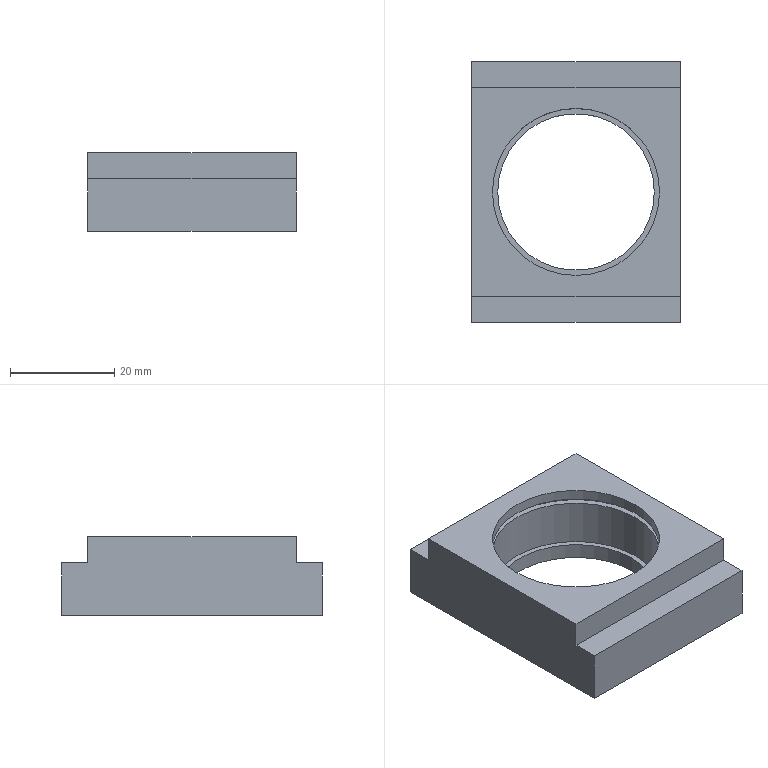Part | STEP file | Bearing fixing seat | 1 solid | 21 faces | box 40 x 50 x 15 mm | volume 16103 mm3 | plane 13 | cylinder 8 | commonest cylinder face diameters 32 x4 30 x2 34.4 x2
STEP:
#1=CARTESIAN_POINT('',(0.,0.,0.));
#2=DIRECTION('',(0.,0.,1.));
#3=DIRECTION('',(1.,0.,0.));
#4=AXIS2_PLACEMENT_3D('',#1,#2,#3);
#5=CARTESIAN_POINT('',(15.,0.,0.));
#6=VERTEX_POINT('',#5);
#7=CARTESIAN_POINT('',(15.,0.,3.));
#8=VERTEX_POINT('',#7);
#9=CARTESIAN_POINT('',(15.,0.,-3.));
#10=DIRECTION('',(0.,0.,1.));
#11=VECTOR('',#10,1.);
#12=LINE('',#9,#11);
#13=CARTESIAN_POINT('',(0.,0.,-3.));
#14=DIRECTION('',(0.,0.,1.));
#15=DIRECTION('',(1.,0.,0.));
#16=AXIS2_PLACEMENT_3D('',#13,#14,#15);
#17=CYLINDRICAL_SURFACE('',#16,15.);
#18=CARTESIAN_POINT('',(6.283,0.));
#19=DIRECTION('',(0.,1.));
#20=VECTOR('',#19,1.);
#21=LINE('',#18,#20);
#22=(GEOMETRIC_REPRESENTATION_CONTEXT(2)PARAMETRIC_REPRESENTATION_CONTEXT()REPRESENTATION_CONTEXT('',''));
#23=DEFINITIONAL_REPRESENTATION('',(#21),#22);
#24=PCURVE('',#17,#23);
#25=CARTESIAN_POINT('',(0.,0.,-3.));
#26=DIRECTION('',(0.,0.,1.));
#27=DIRECTION('',(1.,0.,0.));
#28=AXIS2_PLACEMENT_3D('',#25,#26,#27);
#29=CYLINDRICAL_SURFACE('',#28,15.);
#30=CARTESIAN_POINT('',(0.,0.));
#31=DIRECTION('',(0.,1.));
#32=VECTOR('',#31,1.);
#33=LINE('',#30,#32);
#34=(GEOMETRIC_REPRESENTATION_CONTEXT(2)PARAMETRIC_REPRESENTATION_CONTEXT()REPRESENTATION_CONTEXT('',''));
#35=DEFINITIONAL_REPRESENTATION('',(#33),#34);
#36=PCURVE('',#29,#35);
#37=SURFACE_CURVE('',#12,(#24,#36),.PCURVE_S1.);
#38=EDGE_CURVE('',#6,#8,#37,.T.);
#39=ORIENTED_EDGE('',*,*,#38,.T.);
#40=CARTESIAN_POINT('',(-15.,0.,3.));
#41=VERTEX_POINT('',#40);
#42=CARTESIAN_POINT('',(0.,0.,3.));
#43=DIRECTION('',(0.,0.,-1.));
#44=DIRECTION('',(1.,0.,0.));
#45=AXIS2_PLACEMENT_3D('',#42,#43,#44);
#46=CIRCLE('',#45,15.);
#47=CARTESIAN_POINT('',(6.283,6.));
#48=DIRECTION('',(-1.,0.));
#49=VECTOR('',#48,1.);
#50=LINE('',#47,#49);
#51=(GEOMETRIC_REPRESENTATION_CONTEXT(2)PARAMETRIC_REPRESENTATION_CONTEXT()REPRESENTATION_CONTEXT('',''));
#52=DEFINITIONAL_REPRESENTATION('',(#50),#51);
#53=PCURVE('',#17,#52);
#54=CARTESIAN_POINT('',(0.,0.,3.));
#55=DIRECTION('',(0.,0.,1.));
#56=DIRECTION('',(1.,0.,0.));
#57=AXIS2_PLACEMENT_3D('',#54,#55,#56);
#58=PLANE('',#57);
#59=CARTESIAN_POINT('',(15.,0.));
#60=CARTESIAN_POINT('',(15.,-25.981));
#61=CARTESIAN_POINT('',(-7.5,-12.99));
#62=CARTESIAN_POINT('',(-30.,0.));
#63=CARTESIAN_POINT('',(-7.5,12.99));
#64=CARTESIAN_POINT('',(15.,25.981));
#65=CARTESIAN_POINT('',(15.,0.));
#66=(BOUNDED_CURVE()B_SPLINE_CURVE(2,(#59,#60,#61,#62,#63,#64,#65),.UNSPECIFIED.,.T.,.F.)B_SPLINE_CURVE_WITH_KNOTS((1,2,2,2,2,1),(-2.094,0.,2.094,4.189,6.283,8.378),.UNSPECIFIED.)CURVE()GEOMETRIC_REPRESENTATION_ITEM()RATIONAL_B_SPLINE_CURVE((1.,0.5,1.,0.5,1.,0.5,1.))REPRESENTATION_ITEM(''));
#67=(GEOMETRIC_REPRESENTATION_CONTEXT(2)PARAMETRIC_REPRESENTATION_CONTEXT()REPRESENTATION_CONTEXT('',''));
#68=DEFINITIONAL_REPRESENTATION('',(#66),#67);
#69=PCURVE('',#58,#68);
#70=SURFACE_CURVE('',#46,(#53,#69),.PCURVE_S1.);
#71=EDGE_CURVE('',#8,#41,#70,.T.);
#72=ORIENTED_EDGE('',*,*,#71,.T.);
#73=CARTESIAN_POINT('',(-15.,0.,0.));
#74=VERTEX_POINT('',#73);
#75=CARTESIAN_POINT('',(-15.,0.,-3.));
#76=DIRECTION('',(0.,0.,1.));
#77=VECTOR('',#76,1.);
#78=LINE('',#75,#77);
#79=CARTESIAN_POINT('',(3.142,0.));
#80=DIRECTION('',(0.,1.));
#81=VECTOR('',#80,1.);
#82=LINE('',#79,#81);
#83=(GEOMETRIC_REPRESENTATION_CONTEXT(2)PARAMETRIC_REPRESENTATION_CONTEXT()REPRESENTATION_CONTEXT('',''));
#84=DEFINITIONAL_REPRESENTATION('',(#82),#83);
#85=PCURVE('',#17,#84);
#86=CARTESIAN_POINT('',(3.142,0.));
#87=DIRECTION('',(0.,1.));
#88=VECTOR('',#87,1.);
#89=LINE('',#86,#88);
#90=(GEOMETRIC_REPRESENTATION_CONTEXT(2)PARAMETRIC_REPRESENTATION_CONTEXT()REPRESENTATION_CONTEXT('',''));
#91=DEFINITIONAL_REPRESENTATION('',(#89),#90);
#92=PCURVE('',#29,#91);
#93=SURFACE_CURVE('',#78,(#85,#92),.PCURVE_S1.);
#94=EDGE_CURVE('',#74,#41,#93,.T.);
#95=ORIENTED_EDGE('',*,*,#94,.F.);
#96=CARTESIAN_POINT('',(0.,0.,0.));
#97=DIRECTION('',(0.,0.,-1.));
#98=DIRECTION('',(1.,0.,0.));
#99=AXIS2_PLACEMENT_3D('',#96,#97,#98);
#100=CIRCLE('',#99,15.);
#101=CARTESIAN_POINT('',(6.283,3.));
#102=DIRECTION('',(-1.,0.));
#103=VECTOR('',#102,1.);
#104=LINE('',#101,#103);
#105=(GEOMETRIC_REPRESENTATION_CONTEXT(2)PARAMETRIC_REPRESENTATION_CONTEXT()REPRESENTATION_CONTEXT('',''));
#106=DEFINITIONAL_REPRESENTATION('',(#104),#105);
#107=PCURVE('',#17,#106);
#108=CARTESIAN_POINT('',(0.,0.,0.));
#109=DIRECTION('',(0.,0.,1.));
#110=DIRECTION('',(1.,0.,0.));
#111=AXIS2_PLACEMENT_3D('',#108,#109,#110);
#112=PLANE('',#111);
#113=CARTESIAN_POINT('',(15.,0.));
#114=CARTESIAN_POINT('',(15.,-25.981));
#115=CARTESIAN_POINT('',(-7.5,-12.99));
#116=CARTESIAN_POINT('',(-30.,0.));
#117=CARTESIAN_POINT('',(-7.5,12.99));
#118=CARTESIAN_POINT('',(15.,25.981));
#119=CARTESIAN_POINT('',(15.,0.));
#120=(BOUNDED_CURVE()B_SPLINE_CURVE(2,(#113,#114,#115,#116,#117,#118,#119),.UNSPECIFIED.,.T.,.F.)B_SPLINE_CURVE_WITH_KNOTS((1,2,2,2,2,1),(-2.094,0.,2.094,4.189,6.283,8.378),.UNSPECIFIED.)CURVE()GEOMETRIC_REPRESENTATION_ITEM()RATIONAL_B_SPLINE_CURVE((1.,0.5,1.,0.5,1.,0.5,1.))REPRESENTATION_ITEM(''));
#121=(GEOMETRIC_REPRESENTATION_CONTEXT(2)PARAMETRIC_REPRESENTATION_CONTEXT()REPRESENTATION_CONTEXT('',''));
#122=DEFINITIONAL_REPRESENTATION('',(#120),#121);
#123=PCURVE('',#112,#122);
#124=SURFACE_CURVE('',#100,(#107,#123),.PCURVE_S1.);
#125=EDGE_CURVE('',#6,#74,#124,.T.);
#126=ORIENTED_EDGE('',*,*,#125,.F.);
#127=EDGE_LOOP('',(#39,#72,#95,#126));
#128=FACE_BOUND('',#127,.F.);
#129=ADVANCED_FACE('',(#128),#17,.F.);
#130=CARTESIAN_POINT('',(-16.,0.,15.));
#131=VERTEX_POINT('',#130);
#132=CARTESIAN_POINT('',(-16.,0.,13.));
#133=VERTEX_POINT('',#132);
#134=CARTESIAN_POINT('',(-16.,0.,15.));
#135=DIRECTION('',(0.,0.,-1.));
#136=VECTOR('',#135,1.);
#137=LINE('',#134,#136);
#138=CARTESIAN_POINT('',(0.,0.,15.));
#139=DIRECTION('',(0.,0.,-1.));
#140=DIRECTION('',(-1.,0.,0.));
#141=AXIS2_PLACEMENT_3D('',#138,#139,#140);
#142=CYLINDRICAL_SURFACE('',#141,16.);
#143=CARTESIAN_POINT('',(6.283,0.));
#144=DIRECTION('',(0.,1.));
#145=VECTOR('',#144,1.);
#146=LINE('',#143,#145);
#147=(GEOMETRIC_REPRESENTATION_CONTEXT(2)PARAMETRIC_REPRESENTATION_CONTEXT()REPRESENTATION_CONTEXT('',''));
#148=DEFINITIONAL_REPRESENTATION('',(#146),#147);
#149=PCURVE('',#142,#148);
#150=CARTESIAN_POINT('',(0.,0.,15.));
#151=DIRECTION('',(0.,0.,-1.));
#152=DIRECTION('',(-1.,0.,0.));
#153=AXIS2_PLACEMENT_3D('',#150,#151,#152);
#154=CYLINDRICAL_SURFACE('',#153,16.);
#155=CARTESIAN_POINT('',(0.,0.));
#156=DIRECTION('',(0.,1.));
#157=VECTOR('',#156,1.);
#158=LINE('',#155,#157);
#159=(GEOMETRIC_REPRESENTATION_CONTEXT(2)PARAMETRIC_REPRESENTATION_CONTEXT()REPRESENTATION_CONTEXT('',''));
#160=DEFINITIONAL_REPRESENTATION('',(#158),#159);
#161=PCURVE('',#154,#160);
#162=SURFACE_CURVE('',#137,(#149,#161),.PCURVE_S1.);
#163=EDGE_CURVE('',#131,#133,#162,.T.);
#164=ORIENTED_EDGE('',*,*,#163,.T.);
#165=CARTESIAN_POINT('',(16.,0.,13.));
#166=VERTEX_POINT('',#165);
#167=CARTESIAN_POINT('',(0.,0.,13.));
#168=DIRECTION('',(0.,0.,1.));
#169=DIRECTION('',(-1.,0.,0.));
#170=AXIS2_PLACEMENT_3D('',#167,#168,#169);
#171=CIRCLE('',#170,16.);
#172=CARTESIAN_POINT('',(6.283,2.));
#173=DIRECTION('',(-1.,0.));
#174=VECTOR('',#173,1.);
#175=LINE('',#172,#174);
#176=(GEOMETRIC_REPRESENTATION_CONTEXT(2)PARAMETRIC_REPRESENTATION_CONTEXT()REPRESENTATION_CONTEXT('',''));
#177=DEFINITIONAL_REPRESENTATION('',(#175),#176);
#178=PCURVE('',#142,#177);
#179=CARTESIAN_POINT('',(0.,0.,13.));
#180=DIRECTION('',(0.,0.,1.));
#181=DIRECTION('',(1.,0.,0.));
#182=AXIS2_PLACEMENT_3D('',#179,#180,#181);
#183=PLANE('',#182);
#184=CARTESIAN_POINT('',(0.,0.));
#185=DIRECTION('',(-1.,0.));
#186=AXIS2_PLACEMENT_2D('',#184,#185);
#187=CIRCLE('',#186,16.);
#188=(GEOMETRIC_REPRESENTATION_CONTEXT(2)PARAMETRIC_REPRESENTATION_CONTEXT()REPRESENTATION_CONTEXT('',''));
#189=DEFINITIONAL_REPRESENTATION('',(#187),#188);
#190=PCURVE('',#183,#189);
#191=SURFACE_CURVE('',#171,(#178,#190),.PCURVE_S1.);
#192=EDGE_CURVE('',#133,#166,#191,.T.);
#193=ORIENTED_EDGE('',*,*,#192,.T.);
#194=CARTESIAN_POINT('',(16.,0.,15.));
#195=VERTEX_POINT('',#194);
#196=CARTESIAN_POINT('',(16.,0.,15.));
#197=DIRECTION('',(0.,0.,-1.));
#198=VECTOR('',#197,1.);
#199=LINE('',#196,#198);
#200=CARTESIAN_POINT('',(3.142,0.));
#201=DIRECTION('',(0.,1.));
#202=VECTOR('',#201,1.);
#203=LINE('',#200,#202);
#204=(GEOMETRIC_REPRESENTATION_CONTEXT(2)PARAMETRIC_REPRESENTATION_CONTEXT()REPRESENTATION_CONTEXT('',''));
#205=DEFINITIONAL_REPRESENTATION('',(#203),#204);
#206=PCURVE('',#142,#205);
#207=CARTESIAN_POINT('',(3.142,0.));
#208=DIRECTION('',(0.,1.));
#209=VECTOR('',#208,1.);
#210=LINE('',#207,#209);
#211=(GEOMETRIC_REPRESENTATION_CONTEXT(2)PARAMETRIC_REPRESENTATION_CONTEXT()REPRESENTATION_CONTEXT('',''));
#212=DEFINITIONAL_REPRESENTATION('',(#210),#211);
#213=PCURVE('',#154,#212);
#214=SURFACE_CURVE('',#199,(#206,#213),.PCURVE_S1.);
#215=EDGE_CURVE('',#195,#166,#214,.T.);
#216=ORIENTED_EDGE('',*,*,#215,.F.);
#217=CARTESIAN_POINT('',(0.,0.,15.));
#218=DIRECTION('',(0.,0.,-1.));
#219=DIRECTION('',(-1.,0.,0.));
#220=AXIS2_PLACEMENT_3D('',#217,#218,#219);
#221=CIRCLE('',#220,16.);
#222=CARTESIAN_POINT('',(0.,0.));
#223=DIRECTION('',(1.,0.));
#224=VECTOR('',#223,1.);
#225=LINE('',#222,#224);
#226=(GEOMETRIC_REPRESENTATION_CONTEXT(2)PARAMETRIC_REPRESENTATION_CONTEXT()REPRESENTATION_CONTEXT('',''));
#227=DEFINITIONAL_REPRESENTATION('',(#225),#226);
#228=PCURVE('',#142,#227);
#229=CARTESIAN_POINT('',(0.,0.,15.));
#230=DIRECTION('',(0.,0.,1.));
#231=DIRECTION('',(1.,0.,0.));
#232=AXIS2_PLACEMENT_3D('',#229,#230,#231);
#233=PLANE('',#232);
#234=CARTESIAN_POINT('',(-16.,0.));
#235=CARTESIAN_POINT('',(-16.,27.713));
#236=CARTESIAN_POINT('',(8.,13.856));
#237=CARTESIAN_POINT('',(32.,0.));
#238=CARTESIAN_POINT('',(8.,-13.856));
#239=CARTESIAN_POINT('',(-16.,-27.713));
#240=CARTESIAN_POINT('',(-16.,0.));
#241=(BOUNDED_CURVE()B_SPLINE_CURVE(2,(#234,#235,#236,#237,#238,#239,#240),.UNSPECIFIED.,.T.,.F.)B_SPLINE_CURVE_WITH_KNOTS((1,2,2,2,2,1),(-2.094,0.,2.094,4.189,6.283,8.378),.UNSPECIFIED.)CURVE()GEOMETRIC_REPRESENTATION_ITEM()RATIONAL_B_SPLINE_CURVE((1.,0.5,1.,0.5,1.,0.5,1.))REPRESENTATION_ITEM(''));
#242=(GEOMETRIC_REPRESENTATION_CONTEXT(2)PARAMETRIC_REPRESENTATION_CONTEXT()REPRESENTATION_CONTEXT('',''));
#243=DEFINITIONAL_REPRESENTATION('',(#241),#242);
#244=PCURVE('',#233,#243);
#245=SURFACE_CURVE('',#221,(#228,#244),.PCURVE_S1.);
#246=EDGE_CURVE('',#195,#131,#245,.T.);
#247=ORIENTED_EDGE('',*,*,#246,.T.);
#248=EDGE_LOOP('',(#164,#193,#216,#247));
#249=FACE_BOUND('',#248,.F.);
#250=ADVANCED_FACE('',(#249),#142,.F.);
#251=CARTESIAN_POINT('',(16.,0.,3.));
#252=VERTEX_POINT('',#251);
#253=CARTESIAN_POINT('',(16.,0.,12.));
#254=VERTEX_POINT('',#253);
#255=CARTESIAN_POINT('',(16.,0.,3.));
#256=DIRECTION('',(0.,0.,1.));
#257=VECTOR('',#256,1.);
#258=LINE('',#255,#257);
#259=CARTESIAN_POINT('',(0.,0.,3.));
#260=DIRECTION('',(0.,0.,1.));
#261=DIRECTION('',(1.,0.,0.));
#262=AXIS2_PLACEMENT_3D('',#259,#260,#261);
#263=CYLINDRICAL_SURFACE('',#262,16.);
#264=CARTESIAN_POINT('',(6.283,0.));
#265=DIRECTION('',(0.,1.));
#266=VECTOR('',#265,1.);
#267=LINE('',#264,#266);
#268=(GEOMETRIC_REPRESENTATION_CONTEXT(2)PARAMETRIC_REPRESENTATION_CONTEXT()REPRESENTATION_CONTEXT('',''));
#269=DEFINITIONAL_REPRESENTATION('',(#267),#268);
#270=PCURVE('',#263,#269);
#271=CARTESIAN_POINT('',(0.,0.,3.));
#272=DIRECTION('',(0.,0.,1.));
#273=DIRECTION('',(1.,0.,0.));
#274=AXIS2_PLACEMENT_3D('',#271,#272,#273);
#275=CYLINDRICAL_SURFACE('',#274,16.);
#276=CARTESIAN_POINT('',(0.,0.));
#277=DIRECTION('',(0.,1.));
#278=VECTOR('',#277,1.);
#279=LINE('',#276,#278);
#280=(GEOMETRIC_REPRESENTATION_CONTEXT(2)PARAMETRIC_REPRESENTATION_CONTEXT()REPRESENTATION_CONTEXT('',''));
#281=DEFINITIONAL_REPRESENTATION('',(#279),#280);
#282=PCURVE('',#275,#281);
#283=SURFACE_CURVE('',#258,(#270,#282),.PCURVE_S1.);
#284=EDGE_CURVE('',#252,#254,#283,.T.);
#285=ORIENTED_EDGE('',*,*,#284,.T.);
#286=CARTESIAN_POINT('',(-16.,0.,12.));
#287=VERTEX_POINT('',#286);
#288=CARTESIAN_POINT('',(0.,0.,12.));
#289=DIRECTION('',(0.,0.,-1.));
#290=DIRECTION('',(1.,0.,0.));
#291=AXIS2_PLACEMENT_3D('',#288,#289,#290);
#292=CIRCLE('',#291,16.);
#293=CARTESIAN_POINT('',(6.283,9.));
#294=DIRECTION('',(-1.,0.));
#295=VECTOR('',#294,1.);
#296=LINE('',#293,#295);
#297=(GEOMETRIC_REPRESENTATION_CONTEXT(2)PARAMETRIC_REPRESENTATION_CONTEXT()REPRESENTATION_CONTEXT('',''));
#298=DEFINITIONAL_REPRESENTATION('',(#296),#297);
#299=PCURVE('',#263,#298);
#300=CARTESIAN_POINT('',(0.,0.,12.));
#301=DIRECTION('',(0.,0.,1.));
#302=DIRECTION('',(1.,0.,0.));
#303=AXIS2_PLACEMENT_3D('',#300,#301,#302);
#304=PLANE('',#303);
#305=CARTESIAN_POINT('',(16.,0.));
#306=CARTESIAN_POINT('',(16.,-27.713));
#307=CARTESIAN_POINT('',(-8.,-13.856));
#308=CARTESIAN_POINT('',(-32.,0.));
#309=CARTESIAN_POINT('',(-8.,13.856));
#310=CARTESIAN_POINT('',(16.,27.713));
#311=CARTESIAN_POINT('',(16.,0.));
#312=(BOUNDED_CURVE()B_SPLINE_CURVE(2,(#305,#306,#307,#308,#309,#310,#311),.UNSPECIFIED.,.T.,.F.)B_SPLINE_CURVE_WITH_KNOTS((1,2,2,2,2,1),(-2.094,0.,2.094,4.189,6.283,8.378),.UNSPECIFIED.)CURVE()GEOMETRIC_REPRESENTATION_ITEM()RATIONAL_B_SPLINE_CURVE((1.,0.5,1.,0.5,1.,0.5,1.))REPRESENTATION_ITEM(''));
#313=(GEOMETRIC_REPRESENTATION_CONTEXT(2)PARAMETRIC_REPRESENTATION_CONTEXT()REPRESENTATION_CONTEXT('',''));
#314=DEFINITIONAL_REPRESENTATION('',(#312),#313);
#315=PCURVE('',#304,#314);
#316=SURFACE_CURVE('',#292,(#299,#315),.PCURVE_S1.);
#317=EDGE_CURVE('',#254,#287,#316,.T.);
#318=ORIENTED_EDGE('',*,*,#317,.T.);
#319=CARTESIAN_POINT('',(-16.,0.,3.));
#320=VERTEX_POINT('',#319);
#321=CARTESIAN_POINT('',(-16.,0.,3.));
#322=DIRECTION('',(0.,0.,1.));
#323=VECTOR('',#322,1.);
#324=LINE('',#321,#323);
#325=CARTESIAN_POINT('',(3.142,0.));
#326=DIRECTION('',(0.,1.));
#327=VECTOR('',#326,1.);
#328=LINE('',#325,#327);
#329=(GEOMETRIC_REPRESENTATION_CONTEXT(2)PARAMETRIC_REPRESENTATION_CONTEXT()REPRESENTATION_CONTEXT('',''));
#330=DEFINITIONAL_REPRESENTATION('',(#328),#329);
#331=PCURVE('',#263,#330);
#332=CARTESIAN_POINT('',(3.142,0.));
#333=DIRECTION('',(0.,1.));
#334=VECTOR('',#333,1.);
#335=LINE('',#332,#334);
#336=(GEOMETRIC_REPRESENTATION_CONTEXT(2)PARAMETRIC_REPRESENTATION_CONTEXT()REPRESENTATION_CONTEXT('',''));
#337=DEFINITIONAL_REPRESENTATION('',(#335),#336);
#338=PCURVE('',#275,#337);
#339=SURFACE_CURVE('',#324,(#331,#338),.PCURVE_S1.);
#340=EDGE_CURVE('',#320,#287,#339,.T.);
#341=ORIENTED_EDGE('',*,*,#340,.F.);
#342=CARTESIAN_POINT('',(0.,0.,3.));
#343=DIRECTION('',(0.,0.,1.));
#344=DIRECTION('',(1.,0.,0.));
#345=AXIS2_PLACEMENT_3D('',#342,#343,#344);
#346=CIRCLE('',#345,16.);
#347=CARTESIAN_POINT('',(0.,0.));
#348=DIRECTION('',(1.,0.));
#349=VECTOR('',#348,1.);
#350=LINE('',#347,#349);
#351=(GEOMETRIC_REPRESENTATION_CONTEXT(2)PARAMETRIC_REPRESENTATION_CONTEXT()REPRESENTATION_CONTEXT('',''));
#352=DEFINITIONAL_REPRESENTATION('',(#350),#351);
#353=PCURVE('',#263,#352);
#354=CARTESIAN_POINT('',(0.,0.));
#355=DIRECTION('',(1.,0.));
#356=AXIS2_PLACEMENT_2D('',#354,#355);
#357=CIRCLE('',#356,16.);
#358=(GEOMETRIC_REPRESENTATION_CONTEXT(2)PARAMETRIC_REPRESENTATION_CONTEXT()REPRESENTATION_CONTEXT('',''));
#359=DEFINITIONAL_REPRESENTATION('',(#357),#358);
#360=PCURVE('',#58,#359);
#361=SURFACE_CURVE('',#346,(#353,#360),.PCURVE_S1.);
#362=EDGE_CURVE('',#320,#252,#361,.T.);
#363=ORIENTED_EDGE('',*,*,#362,.T.);
#364=EDGE_LOOP('',(#285,#318,#341,#363));
#365=FACE_BOUND('',#364,.F.);
#366=ADVANCED_FACE('',(#365),#263,.F.);
#367=CARTESIAN_POINT('',(-17.2,0.,13.));
#368=VERTEX_POINT('',#367);
#369=CARTESIAN_POINT('',(-17.2,0.,12.));
#370=VERTEX_POINT('',#369);
#371=CARTESIAN_POINT('',(-17.2,0.,13.));
#372=DIRECTION('',(0.,0.,-1.));
#373=VECTOR('',#372,1.);
#374=LINE('',#371,#373);
#375=CARTESIAN_POINT('',(0.,0.,13.));
#376=DIRECTION('',(0.,0.,-1.));
#377=DIRECTION('',(-1.,0.,0.));
#378=AXIS2_PLACEMENT_3D('',#375,#376,#377);
#379=CYLINDRICAL_SURFACE('',#378,17.2);
#380=CARTESIAN_POINT('',(6.283,0.));
#381=DIRECTION('',(0.,1.));
#382=VECTOR('',#381,1.);
#383=LINE('',#380,#382);
#384=(GEOMETRIC_REPRESENTATION_CONTEXT(2)PARAMETRIC_REPRESENTATION_CONTEXT()REPRESENTATION_CONTEXT('',''));
#385=DEFINITIONAL_REPRESENTATION('',(#383),#384);
#386=PCURVE('',#379,#385);
#387=CARTESIAN_POINT('',(0.,0.,13.));
#388=DIRECTION('',(0.,0.,-1.));
#389=DIRECTION('',(-1.,0.,0.));
#390=AXIS2_PLACEMENT_3D('',#387,#388,#389);
#391=CYLINDRICAL_SURFACE('',#390,17.2);
#392=CARTESIAN_POINT('',(0.,0.));
#393=DIRECTION('',(0.,1.));
#394=VECTOR('',#393,1.);
#395=LINE('',#392,#394);
#396=(GEOMETRIC_REPRESENTATION_CONTEXT(2)PARAMETRIC_REPRESENTATION_CONTEXT()REPRESENTATION_CONTEXT('',''));
#397=DEFINITIONAL_REPRESENTATION('',(#395),#396);
#398=PCURVE('',#391,#397);
#399=SURFACE_CURVE('',#374,(#386,#398),.PCURVE_S1.);
#400=EDGE_CURVE('',#368,#370,#399,.T.);
#401=ORIENTED_EDGE('',*,*,#400,.T.);
#402=CARTESIAN_POINT('',(17.2,0.,12.));
#403=VERTEX_POINT('',#402);
#404=CARTESIAN_POINT('',(0.,0.,12.));
#405=DIRECTION('',(0.,0.,1.));
#406=DIRECTION('',(-1.,0.,0.));
#407=AXIS2_PLACEMENT_3D('',#404,#405,#406);
#408=CIRCLE('',#407,17.2);
#409=CARTESIAN_POINT('',(6.283,1.));
#410=DIRECTION('',(-1.,0.));
#411=VECTOR('',#410,1.);
#412=LINE('',#409,#411);
#413=(GEOMETRIC_REPRESENTATION_CONTEXT(2)PARAMETRIC_REPRESENTATION_CONTEXT()REPRESENTATION_CONTEXT('',''));
#414=DEFINITIONAL_REPRESENTATION('',(#412),#413);
#415=PCURVE('',#379,#414);
#416=CARTESIAN_POINT('',(0.,0.));
#417=DIRECTION('',(-1.,0.));
#418=AXIS2_PLACEMENT_2D('',#416,#417);
#419=CIRCLE('',#418,17.2);
#420=(GEOMETRIC_REPRESENTATION_CONTEXT(2)PARAMETRIC_REPRESENTATION_CONTEXT()REPRESENTATION_CONTEXT('',''));
#421=DEFINITIONAL_REPRESENTATION('',(#419),#420);
#422=PCURVE('',#304,#421);
#423=SURFACE_CURVE('',#408,(#415,#422),.PCURVE_S1.);
#424=EDGE_CURVE('',#370,#403,#423,.T.);
#425=ORIENTED_EDGE('',*,*,#424,.T.);
#426=CARTESIAN_POINT('',(17.2,0.,13.));
#427=VERTEX_POINT('',#426);
#428=CARTESIAN_POINT('',(17.2,0.,13.));
#429=DIRECTION('',(0.,0.,-1.));
#430=VECTOR('',#429,1.);
#431=LINE('',#428,#430);
#432=CARTESIAN_POINT('',(3.142,0.));
#433=DIRECTION('',(0.,1.));
#434=VECTOR('',#433,1.);
#435=LINE('',#432,#434);
#436=(GEOMETRIC_REPRESENTATION_CONTEXT(2)PARAMETRIC_REPRESENTATION_CONTEXT()REPRESENTATION_CONTEXT('',''));
#437=DEFINITIONAL_REPRESENTATION('',(#435),#436);
#438=PCURVE('',#379,#437);
#439=CARTESIAN_POINT('',(3.142,0.));
#440=DIRECTION('',(0.,1.));
#441=VECTOR('',#440,1.);
#442=LINE('',#439,#441);
#443=(GEOMETRIC_REPRESENTATION_CONTEXT(2)PARAMETRIC_REPRESENTATION_CONTEXT()REPRESENTATION_CONTEXT('',''));
#444=DEFINITIONAL_REPRESENTATION('',(#442),#443);
#445=PCURVE('',#391,#444);
#446=SURFACE_CURVE('',#431,(#438,#445),.PCURVE_S1.);
#447=EDGE_CURVE('',#427,#403,#446,.T.);
#448=ORIENTED_EDGE('',*,*,#447,.F.);
#449=CARTESIAN_POINT('',(0.,0.,13.));
#450=DIRECTION('',(0.,0.,1.));
#451=DIRECTION('',(-1.,0.,0.));
#452=AXIS2_PLACEMENT_3D('',#449,#450,#451);
#453=CIRCLE('',#452,17.2);
#454=CARTESIAN_POINT('',(6.283,0.));
#455=DIRECTION('',(-1.,0.));
#456=VECTOR('',#455,1.);
#457=LINE('',#454,#456);
#458=(GEOMETRIC_REPRESENTATION_CONTEXT(2)PARAMETRIC_REPRESENTATION_CONTEXT()REPRESENTATION_CONTEXT('',''));
#459=DEFINITIONAL_REPRESENTATION('',(#457),#458);
#460=PCURVE('',#379,#459);
#461=CARTESIAN_POINT('',(0.,0.));
#462=DIRECTION('',(-1.,0.));
#463=AXIS2_PLACEMENT_2D('',#461,#462);
#464=CIRCLE('',#463,17.2);
#465=(GEOMETRIC_REPRESENTATION_CONTEXT(2)PARAMETRIC_REPRESENTATION_CONTEXT()REPRESENTATION_CONTEXT('',''));
#466=DEFINITIONAL_REPRESENTATION('',(#464),#465);
#467=PCURVE('',#183,#466);
#468=SURFACE_CURVE('',#453,(#460,#467),.PCURVE_S1.);
#469=EDGE_CURVE('',#368,#427,#468,.T.);
#470=ORIENTED_EDGE('',*,*,#469,.F.);
#471=EDGE_LOOP('',(#401,#425,#448,#470));
#472=FACE_BOUND('',#471,.F.);
#473=ADVANCED_FACE('',(#472),#379,.F.);
#474=CARTESIAN_POINT('',(-20.,-25.,0.));
#475=VERTEX_POINT('',#474);
#476=CARTESIAN_POINT('',(20.,-25.,0.));
#477=VERTEX_POINT('',#476);
#478=CARTESIAN_POINT('',(0.,-25.,0.));
#479=DIRECTION('',(1.,0.,0.));
#480=VECTOR('',#479,1.);
#481=LINE('',#478,#480);
#482=CARTESIAN_POINT('',(0.,-25.));
#483=DIRECTION('',(1.,0.));
#484=VECTOR('',#483,1.);
#485=LINE('',#482,#484);
#486=(GEOMETRIC_REPRESENTATION_CONTEXT(2)PARAMETRIC_REPRESENTATION_CONTEXT()REPRESENTATION_CONTEXT('',''));
#487=DEFINITIONAL_REPRESENTATION('',(#485),#486);
#488=PCURVE('',#112,#487);
#489=CARTESIAN_POINT('',(20.,-25.,10.));
#490=DIRECTION('',(0.,-1.,0.));
#491=DIRECTION('',(0.,0.,-1.));
#492=AXIS2_PLACEMENT_3D('',#489,#490,#491);
#493=PLANE('',#492);
#494=CARTESIAN_POINT('',(10.,-20.));
#495=DIRECTION('',(0.,1.));
#496=VECTOR('',#495,1.);
#497=LINE('',#494,#496);
#498=(GEOMETRIC_REPRESENTATION_CONTEXT(2)PARAMETRIC_REPRESENTATION_CONTEXT()REPRESENTATION_CONTEXT('',''));
#499=DEFINITIONAL_REPRESENTATION('',(#497),#498);
#500=PCURVE('',#493,#499);
#501=SURFACE_CURVE('',#481,(#488,#500),.PCURVE_S1.);
#502=EDGE_CURVE('',#475,#477,#501,.T.);
#503=ORIENTED_EDGE('',*,*,#502,.F.);
#504=CARTESIAN_POINT('',(-20.,25.,0.));
#505=VERTEX_POINT('',#504);
#506=CARTESIAN_POINT('',(-20.,0.,0.));
#507=DIRECTION('',(0.,-1.,0.));
#508=VECTOR('',#507,1.);
#509=LINE('',#506,#508);
#510=CARTESIAN_POINT('',(-20.,0.));
#511=DIRECTION('',(0.,-1.));
#512=VECTOR('',#511,1.);
#513=LINE('',#510,#512);
#514=(GEOMETRIC_REPRESENTATION_CONTEXT(2)PARAMETRIC_REPRESENTATION_CONTEXT()REPRESENTATION_CONTEXT('',''));
#515=DEFINITIONAL_REPRESENTATION('',(#513),#514);
#516=PCURVE('',#112,#515);
#517=CARTESIAN_POINT('',(-20.,20.,12.));
#518=DIRECTION('',(1.,0.,0.));
#519=DIRECTION('',(0.,1.,0.));
#520=AXIS2_PLACEMENT_3D('',#517,#518,#519);
#521=PLANE('',#520);
#522=CARTESIAN_POINT('',(-20.,-12.));
#523=DIRECTION('',(-1.,0.));
#524=VECTOR('',#523,1.);
#525=LINE('',#522,#524);
#526=(GEOMETRIC_REPRESENTATION_CONTEXT(2)PARAMETRIC_REPRESENTATION_CONTEXT()REPRESENTATION_CONTEXT('',''));
#527=DEFINITIONAL_REPRESENTATION('',(#525),#526);
#528=PCURVE('',#521,#527);
#529=SURFACE_CURVE('',#509,(#516,#528),.PCURVE_S1.);
#530=EDGE_CURVE('',#505,#475,#529,.T.);
#531=ORIENTED_EDGE('',*,*,#530,.F.);
#532=CARTESIAN_POINT('',(20.,25.,0.));
#533=VERTEX_POINT('',#532);
#534=CARTESIAN_POINT('',(0.,25.,0.));
#535=DIRECTION('',(-1.,0.,0.));
#536=VECTOR('',#535,1.);
#537=LINE('',#534,#536);
#538=CARTESIAN_POINT('',(0.,25.));
#539=DIRECTION('',(-1.,0.));
#540=VECTOR('',#539,1.);
#541=LINE('',#538,#540);
#542=(GEOMETRIC_REPRESENTATION_CONTEXT(2)PARAMETRIC_REPRESENTATION_CONTEXT()REPRESENTATION_CONTEXT('',''));
#543=DEFINITIONAL_REPRESENTATION('',(#541),#542);
#544=PCURVE('',#112,#543);
#545=CARTESIAN_POINT('',(20.,25.,10.));
#546=DIRECTION('',(0.,1.,0.));
#547=DIRECTION('',(0.,0.,1.));
#548=AXIS2_PLACEMENT_3D('',#545,#546,#547);
#549=PLANE('',#548);
#550=CARTESIAN_POINT('',(-10.,-20.));
#551=DIRECTION('',(0.,-1.));
#552=VECTOR('',#551,1.);
#553=LINE('',#550,#552);
#554=(GEOMETRIC_REPRESENTATION_CONTEXT(2)PARAMETRIC_REPRESENTATION_CONTEXT()REPRESENTATION_CONTEXT('',''));
#555=DEFINITIONAL_REPRESENTATION('',(#553),#554);
#556=PCURVE('',#549,#555);
#557=SURFACE_CURVE('',#537,(#544,#556),.PCURVE_S1.);
#558=EDGE_CURVE('',#533,#505,#557,.T.);
#559=ORIENTED_EDGE('',*,*,#558,.F.);
#560=CARTESIAN_POINT('',(20.,0.,0.));
#561=DIRECTION('',(0.,1.,0.));
#562=VECTOR('',#561,1.);
#563=LINE('',#560,#562);
#564=CARTESIAN_POINT('',(20.,0.));
#565=DIRECTION('',(0.,1.));
#566=VECTOR('',#565,1.);
#567=LINE('',#564,#566);
#568=(GEOMETRIC_REPRESENTATION_CONTEXT(2)PARAMETRIC_REPRESENTATION_CONTEXT()REPRESENTATION_CONTEXT('',''));
#569=DEFINITIONAL_REPRESENTATION('',(#567),#568);
#570=PCURVE('',#112,#569);
#571=CARTESIAN_POINT('',(20.,20.,12.));
#572=DIRECTION('',(-1.,0.,0.));
#573=DIRECTION('',(0.,-1.,0.));
#574=AXIS2_PLACEMENT_3D('',#571,#572,#573);
#575=PLANE('',#574);
#576=CARTESIAN_POINT('',(20.,-12.));
#577=DIRECTION('',(-1.,0.));
#578=VECTOR('',#577,1.);
#579=LINE('',#576,#578);
#580=(GEOMETRIC_REPRESENTATION_CONTEXT(2)PARAMETRIC_REPRESENTATION_CONTEXT()REPRESENTATION_CONTEXT('',''));
#581=DEFINITIONAL_REPRESENTATION('',(#579),#580);
#582=PCURVE('',#575,#581);
#583=SURFACE_CURVE('',#563,(#570,#582),.PCURVE_S1.);
#584=EDGE_CURVE('',#477,#533,#583,.T.);
#585=ORIENTED_EDGE('',*,*,#584,.F.);
#586=EDGE_LOOP('',(#503,#531,#559,#585));
#587=FACE_BOUND('',#586,.T.);
#588=ORIENTED_EDGE('',*,*,#125,.F.);
#589=CARTESIAN_POINT('',(0.,0.,0.));
#590=DIRECTION('',(0.,0.,-1.));
#591=DIRECTION('',(1.,0.,0.));
#592=AXIS2_PLACEMENT_3D('',#589,#590,#591);
#593=CIRCLE('',#592,15.);
#594=CARTESIAN_POINT('',(15.,0.));
#595=CARTESIAN_POINT('',(15.,-25.981));
#596=CARTESIAN_POINT('',(-7.5,-12.99));
#597=CARTESIAN_POINT('',(-30.,0.));
#598=CARTESIAN_POINT('',(-7.5,12.99));
#599=CARTESIAN_POINT('',(15.,25.981));
#600=CARTESIAN_POINT('',(15.,0.));
#601=(BOUNDED_CURVE()B_SPLINE_CURVE(2,(#594,#595,#596,#597,#598,#599,#600),.UNSPECIFIED.,.T.,.F.)B_SPLINE_CURVE_WITH_KNOTS((1,2,2,2,2,1),(-2.094,0.,2.094,4.189,6.283,8.378),.UNSPECIFIED.)CURVE()GEOMETRIC_REPRESENTATION_ITEM()RATIONAL_B_SPLINE_CURVE((1.,0.5,1.,0.5,1.,0.5,1.))REPRESENTATION_ITEM(''));
#602=(GEOMETRIC_REPRESENTATION_CONTEXT(2)PARAMETRIC_REPRESENTATION_CONTEXT()REPRESENTATION_CONTEXT('',''));
#603=DEFINITIONAL_REPRESENTATION('',(#601),#602);
#604=PCURVE('',#112,#603);
#605=CARTESIAN_POINT('',(6.283,3.));
#606=DIRECTION('',(-1.,0.));
#607=VECTOR('',#606,1.);
#608=LINE('',#605,#607);
#609=(GEOMETRIC_REPRESENTATION_CONTEXT(2)PARAMETRIC_REPRESENTATION_CONTEXT()REPRESENTATION_CONTEXT('',''));
#610=DEFINITIONAL_REPRESENTATION('',(#608),#609);
#611=PCURVE('',#29,#610);
#612=SURFACE_CURVE('',#593,(#604,#611),.PCURVE_S1.);
#613=EDGE_CURVE('',#74,#6,#612,.T.);
#614=ORIENTED_EDGE('',*,*,#613,.F.);
#615=EDGE_LOOP('',(#588,#614));
#616=FACE_BOUND('',#615,.T.);
#617=ADVANCED_FACE('',(#587,#616),#112,.F.);
#618=CARTESIAN_POINT('',(20.,25.,10.));
#619=VERTEX_POINT('',#618);
#620=CARTESIAN_POINT('',(20.,25.,12.));
#621=DIRECTION('',(0.,0.,-1.));
#622=VECTOR('',#621,1.);
#623=LINE('',#620,#622);
#624=CARTESIAN_POINT('',(-5.,0.));
#625=DIRECTION('',(0.,-1.));
#626=VECTOR('',#625,1.);
#627=LINE('',#624,#626);
#628=(GEOMETRIC_REPRESENTATION_CONTEXT(2)PARAMETRIC_REPRESENTATION_CONTEXT()REPRESENTATION_CONTEXT('',''));
#629=DEFINITIONAL_REPRESENTATION('',(#627),#628);
#630=PCURVE('',#575,#629);
#631=CARTESIAN_POINT('',(2.,0.));
#632=DIRECTION('',(-1.,0.));
#633=VECTOR('',#632,1.);
#634=LINE('',#631,#633);
#635=(GEOMETRIC_REPRESENTATION_CONTEXT(2)PARAMETRIC_REPRESENTATION_CONTEXT()REPRESENTATION_CONTEXT('',''));
#636=DEFINITIONAL_REPRESENTATION('',(#634),#635);
#637=PCURVE('',#549,#636);
#638=SURFACE_CURVE('',#623,(#630,#637),.PCURVE_S1.);
#639=EDGE_CURVE('',#619,#533,#638,.T.);
#640=ORIENTED_EDGE('',*,*,#639,.F.);
#641=CARTESIAN_POINT('',(20.,20.,10.));
#642=VERTEX_POINT('',#641);
#643=CARTESIAN_POINT('',(20.,20.,10.));
#644=DIRECTION('',(0.,1.,0.));
#645=VECTOR('',#644,1.);
#646=LINE('',#643,#645);
#647=CARTESIAN_POINT('',(0.,-2.));
#648=DIRECTION('',(-1.,0.));
#649=VECTOR('',#648,1.);
#650=LINE('',#647,#649);
#651=(GEOMETRIC_REPRESENTATION_CONTEXT(2)PARAMETRIC_REPRESENTATION_CONTEXT()REPRESENTATION_CONTEXT('',''));
#652=DEFINITIONAL_REPRESENTATION('',(#650),#651);
#653=PCURVE('',#575,#652);
#654=CARTESIAN_POINT('',(0.,0.,10.));
#655=DIRECTION('',(0.,0.,1.));
#656=DIRECTION('',(1.,0.,0.));
#657=AXIS2_PLACEMENT_3D('',#654,#655,#656);
#658=PLANE('',#657);
#659=CARTESIAN_POINT('',(20.,20.));
#660=DIRECTION('',(0.,1.));
#661=VECTOR('',#660,1.);
#662=LINE('',#659,#661);
#663=(GEOMETRIC_REPRESENTATION_CONTEXT(2)PARAMETRIC_REPRESENTATION_CONTEXT()REPRESENTATION_CONTEXT('',''));
#664=DEFINITIONAL_REPRESENTATION('',(#662),#663);
#665=PCURVE('',#658,#664);
#666=SURFACE_CURVE('',#646,(#653,#665),.PCURVE_S1.);
#667=EDGE_CURVE('',#642,#619,#666,.T.);
#668=ORIENTED_EDGE('',*,*,#667,.F.);
#669=CARTESIAN_POINT('',(20.,20.,15.));
#670=VERTEX_POINT('',#669);
#671=CARTESIAN_POINT('',(20.,20.,12.));
#672=DIRECTION('',(0.,0.,-1.));
#673=VECTOR('',#672,1.);
#674=LINE('',#671,#673);
#675=CARTESIAN_POINT('',(0.,0.));
#676=DIRECTION('',(0.,-1.));
#677=VECTOR('',#676,1.);
#678=LINE('',#675,#677);
#679=(GEOMETRIC_REPRESENTATION_CONTEXT(2)PARAMETRIC_REPRESENTATION_CONTEXT()REPRESENTATION_CONTEXT('',''));
#680=DEFINITIONAL_REPRESENTATION('',(#678),#679);
#681=PCURVE('',#575,#680);
#682=CARTESIAN_POINT('',(-20.,20.,12.));
#683=DIRECTION('',(0.,-1.,0.));
#684=DIRECTION('',(0.,0.,-1.));
#685=AXIS2_PLACEMENT_3D('',#682,#683,#684);
#686=PLANE('',#685);
#687=CARTESIAN_POINT('',(0.,40.));
#688=DIRECTION('',(1.,0.));
#689=VECTOR('',#688,1.);
#690=LINE('',#687,#689);
#691=(GEOMETRIC_REPRESENTATION_CONTEXT(2)PARAMETRIC_REPRESENTATION_CONTEXT()REPRESENTATION_CONTEXT('',''));
#692=DEFINITIONAL_REPRESENTATION('',(#690),#691);
#693=PCURVE('',#686,#692);
#694=SURFACE_CURVE('',#674,(#681,#693),.PCURVE_S1.);
#695=EDGE_CURVE('',#670,#642,#694,.T.);
#696=ORIENTED_EDGE('',*,*,#695,.F.);
#697=CARTESIAN_POINT('',(20.,-20.,15.));
#698=VERTEX_POINT('',#697);
#699=CARTESIAN_POINT('',(20.,20.,15.));
#700=DIRECTION('',(0.,1.,0.));
#701=VECTOR('',#700,1.);
#702=LINE('',#699,#701);
#703=CARTESIAN_POINT('',(0.,3.));
#704=DIRECTION('',(-1.,0.));
#705=VECTOR('',#704,1.);
#706=LINE('',#703,#705);
#707=(GEOMETRIC_REPRESENTATION_CONTEXT(2)PARAMETRIC_REPRESENTATION_CONTEXT()REPRESENTATION_CONTEXT('',''));
#708=DEFINITIONAL_REPRESENTATION('',(#706),#707);
#709=PCURVE('',#575,#708);
#710=CARTESIAN_POINT('',(20.,20.));
#711=DIRECTION('',(0.,1.));
#712=VECTOR('',#711,1.);
#713=LINE('',#710,#712);
#714=(GEOMETRIC_REPRESENTATION_CONTEXT(2)PARAMETRIC_REPRESENTATION_CONTEXT()REPRESENTATION_CONTEXT('',''));
#715=DEFINITIONAL_REPRESENTATION('',(#713),#714);
#716=PCURVE('',#233,#715);
#717=SURFACE_CURVE('',#702,(#709,#716),.PCURVE_S1.);
#718=EDGE_CURVE('',#698,#670,#717,.T.);
#719=ORIENTED_EDGE('',*,*,#718,.F.);
#720=CARTESIAN_POINT('',(20.,-20.,10.));
#721=VERTEX_POINT('',#720);
#722=CARTESIAN_POINT('',(20.,-20.,12.));
#723=DIRECTION('',(0.,0.,1.));
#724=VECTOR('',#723,1.);
#725=LINE('',#722,#724);
#726=CARTESIAN_POINT('',(40.,0.));
#727=DIRECTION('',(0.,1.));
#728=VECTOR('',#727,1.);
#729=LINE('',#726,#728);
#730=(GEOMETRIC_REPRESENTATION_CONTEXT(2)PARAMETRIC_REPRESENTATION_CONTEXT()REPRESENTATION_CONTEXT('',''));
#731=DEFINITIONAL_REPRESENTATION('',(#729),#730);
#732=PCURVE('',#575,#731);
#733=CARTESIAN_POINT('',(-20.,-20.,12.));
#734=DIRECTION('',(0.,1.,0.));
#735=DIRECTION('',(0.,0.,1.));
#736=AXIS2_PLACEMENT_3D('',#733,#734,#735);
#737=PLANE('',#736);
#738=CARTESIAN_POINT('',(0.,40.));
#739=DIRECTION('',(1.,0.));
#740=VECTOR('',#739,1.);
#741=LINE('',#738,#740);
#742=(GEOMETRIC_REPRESENTATION_CONTEXT(2)PARAMETRIC_REPRESENTATION_CONTEXT()REPRESENTATION_CONTEXT('',''));
#743=DEFINITIONAL_REPRESENTATION('',(#741),#742);
#744=PCURVE('',#737,#743);
#745=SURFACE_CURVE('',#725,(#732,#744),.PCURVE_S1.);
#746=EDGE_CURVE('',#721,#698,#745,.T.);
#747=ORIENTED_EDGE('',*,*,#746,.F.);
#748=CARTESIAN_POINT('',(20.,-25.,10.));
#749=VERTEX_POINT('',#748);
#750=CARTESIAN_POINT('',(20.,20.,10.));
#751=DIRECTION('',(0.,1.,0.));
#752=VECTOR('',#751,1.);
#753=LINE('',#750,#752);
#754=CARTESIAN_POINT('',(0.,-2.));
#755=DIRECTION('',(-1.,0.));
#756=VECTOR('',#755,1.);
#757=LINE('',#754,#756);
#758=(GEOMETRIC_REPRESENTATION_CONTEXT(2)PARAMETRIC_REPRESENTATION_CONTEXT()REPRESENTATION_CONTEXT('',''));
#759=DEFINITIONAL_REPRESENTATION('',(#757),#758);
#760=PCURVE('',#575,#759);
#761=CARTESIAN_POINT('',(0.,0.,10.));
#762=DIRECTION('',(0.,0.,-1.));
#763=DIRECTION('',(-1.,0.,0.));
#764=AXIS2_PLACEMENT_3D('',#761,#762,#763);
#765=PLANE('',#764);
#766=CARTESIAN_POINT('',(-20.,20.));
#767=DIRECTION('',(0.,1.));
#768=VECTOR('',#767,1.);
#769=LINE('',#766,#768);
#770=(GEOMETRIC_REPRESENTATION_CONTEXT(2)PARAMETRIC_REPRESENTATION_CONTEXT()REPRESENTATION_CONTEXT('',''));
#771=DEFINITIONAL_REPRESENTATION('',(#769),#770);
#772=PCURVE('',#765,#771);
#773=SURFACE_CURVE('',#753,(#760,#772),.PCURVE_S1.);
#774=EDGE_CURVE('',#749,#721,#773,.T.);
#775=ORIENTED_EDGE('',*,*,#774,.F.);
#776=CARTESIAN_POINT('',(20.,-25.,12.));
#777=DIRECTION('',(0.,0.,1.));
#778=VECTOR('',#777,1.);
#779=LINE('',#776,#778);
#780=CARTESIAN_POINT('',(45.,0.));
#781=DIRECTION('',(0.,1.));
#782=VECTOR('',#781,1.);
#783=LINE('',#780,#782);
#784=(GEOMETRIC_REPRESENTATION_CONTEXT(2)PARAMETRIC_REPRESENTATION_CONTEXT()REPRESENTATION_CONTEXT('',''));
#785=DEFINITIONAL_REPRESENTATION('',(#783),#784);
#786=PCURVE('',#575,#785);
#787=CARTESIAN_POINT('',(-2.,0.));
#788=DIRECTION('',(-1.,0.));
#789=VECTOR('',#788,1.);
#790=LINE('',#787,#789);
#791=(GEOMETRIC_REPRESENTATION_CONTEXT(2)PARAMETRIC_REPRESENTATION_CONTEXT()REPRESENTATION_CONTEXT('',''));
#792=DEFINITIONAL_REPRESENTATION('',(#790),#791);
#793=PCURVE('',#493,#792);
#794=SURFACE_CURVE('',#779,(#786,#793),.PCURVE_S1.);
#795=EDGE_CURVE('',#477,#749,#794,.T.);
#796=ORIENTED_EDGE('',*,*,#795,.F.);
#797=ORIENTED_EDGE('',*,*,#584,.T.);
#798=EDGE_LOOP('',(#640,#668,#696,#719,#747,#775,#796,#797));
#799=FACE_BOUND('',#798,.T.);
#800=ADVANCED_FACE('',(#799),#575,.F.);
#801=CARTESIAN_POINT('',(-20.,-25.,10.));
#802=VERTEX_POINT('',#801);
#803=CARTESIAN_POINT('',(20.,-25.,10.));
#804=DIRECTION('',(-1.,0.,0.));
#805=VECTOR('',#804,1.);
#806=LINE('',#803,#805);
#807=CARTESIAN_POINT('',(0.,0.));
#808=DIRECTION('',(0.,-1.));
#809=VECTOR('',#808,1.);
#810=LINE('',#807,#809);
#811=(GEOMETRIC_REPRESENTATION_CONTEXT(2)PARAMETRIC_REPRESENTATION_CONTEXT()REPRESENTATION_CONTEXT('',''));
#812=DEFINITIONAL_REPRESENTATION('',(#810),#811);
#813=PCURVE('',#493,#812);
#814=CARTESIAN_POINT('',(-20.,-25.));
#815=DIRECTION('',(1.,0.));
#816=VECTOR('',#815,1.);
#817=LINE('',#814,#816);
#818=(GEOMETRIC_REPRESENTATION_CONTEXT(2)PARAMETRIC_REPRESENTATION_CONTEXT()REPRESENTATION_CONTEXT('',''));
#819=DEFINITIONAL_REPRESENTATION('',(#817),#818);
#820=PCURVE('',#765,#819);
#821=SURFACE_CURVE('',#806,(#813,#820),.PCURVE_S1.);
#822=EDGE_CURVE('',#749,#802,#821,.T.);
#823=ORIENTED_EDGE('',*,*,#822,.T.);
#824=CARTESIAN_POINT('',(-20.,-25.,10.));
#825=DIRECTION('',(0.,0.,-1.));
#826=VECTOR('',#825,1.);
#827=LINE('',#824,#826);
#828=CARTESIAN_POINT('',(0.,-40.));
#829=DIRECTION('',(1.,0.));
#830=VECTOR('',#829,1.);
#831=LINE('',#828,#830);
#832=(GEOMETRIC_REPRESENTATION_CONTEXT(2)PARAMETRIC_REPRESENTATION_CONTEXT()REPRESENTATION_CONTEXT('',''));
#833=DEFINITIONAL_REPRESENTATION('',(#831),#832);
#834=PCURVE('',#493,#833);
#835=CARTESIAN_POINT('',(-45.,-2.));
#836=DIRECTION('',(0.,-1.));
#837=VECTOR('',#836,1.);
#838=LINE('',#835,#837);
#839=(GEOMETRIC_REPRESENTATION_CONTEXT(2)PARAMETRIC_REPRESENTATION_CONTEXT()REPRESENTATION_CONTEXT('',''));
#840=DEFINITIONAL_REPRESENTATION('',(#838),#839);
#841=PCURVE('',#521,#840);
#842=SURFACE_CURVE('',#827,(#834,#841),.PCURVE_S1.);
#843=EDGE_CURVE('',#802,#475,#842,.T.);
#844=ORIENTED_EDGE('',*,*,#843,.T.);
#845=ORIENTED_EDGE('',*,*,#502,.T.);
#846=ORIENTED_EDGE('',*,*,#795,.T.);
#847=EDGE_LOOP('',(#823,#844,#845,#846));
#848=FACE_BOUND('',#847,.T.);
#849=ADVANCED_FACE('',(#848),#493,.T.);
#850=ORIENTED_EDGE('',*,*,#843,.F.);
#851=CARTESIAN_POINT('',(-20.,-20.,10.));
#852=VERTEX_POINT('',#851);
#853=CARTESIAN_POINT('',(-20.,20.,10.));
#854=DIRECTION('',(0.,-1.,0.));
#855=VECTOR('',#854,1.);
#856=LINE('',#853,#855);
#857=CARTESIAN_POINT('',(0.,-2.));
#858=DIRECTION('',(-1.,0.));
#859=VECTOR('',#858,1.);
#860=LINE('',#857,#859);
#861=(GEOMETRIC_REPRESENTATION_CONTEXT(2)PARAMETRIC_REPRESENTATION_CONTEXT()REPRESENTATION_CONTEXT('',''));
#862=DEFINITIONAL_REPRESENTATION('',(#860),#861);
#863=PCURVE('',#521,#862);
#864=CARTESIAN_POINT('',(20.,20.));
#865=DIRECTION('',(0.,-1.));
#866=VECTOR('',#865,1.);
#867=LINE('',#864,#866);
#868=(GEOMETRIC_REPRESENTATION_CONTEXT(2)PARAMETRIC_REPRESENTATION_CONTEXT()REPRESENTATION_CONTEXT('',''));
#869=DEFINITIONAL_REPRESENTATION('',(#867),#868);
#870=PCURVE('',#765,#869);
#871=SURFACE_CURVE('',#856,(#863,#870),.PCURVE_S1.);
#872=EDGE_CURVE('',#852,#802,#871,.T.);
#873=ORIENTED_EDGE('',*,*,#872,.F.);
#874=CARTESIAN_POINT('',(-20.,-20.,15.));
#875=VERTEX_POINT('',#874);
#876=CARTESIAN_POINT('',(-20.,-20.,12.));
#877=DIRECTION('',(0.,0.,-1.));
#878=VECTOR('',#877,1.);
#879=LINE('',#876,#878);
#880=CARTESIAN_POINT('',(-40.,0.));
#881=DIRECTION('',(0.,-1.));
#882=VECTOR('',#881,1.);
#883=LINE('',#880,#882);
#884=(GEOMETRIC_REPRESENTATION_CONTEXT(2)PARAMETRIC_REPRESENTATION_CONTEXT()REPRESENTATION_CONTEXT('',''));
#885=DEFINITIONAL_REPRESENTATION('',(#883),#884);
#886=PCURVE('',#521,#885);
#887=CARTESIAN_POINT('',(0.,0.));
#888=DIRECTION('',(-1.,0.));
#889=VECTOR('',#888,1.);
#890=LINE('',#887,#889);
#891=(GEOMETRIC_REPRESENTATION_CONTEXT(2)PARAMETRIC_REPRESENTATION_CONTEXT()REPRESENTATION_CONTEXT('',''));
#892=DEFINITIONAL_REPRESENTATION('',(#890),#891);
#893=PCURVE('',#737,#892);
#894=SURFACE_CURVE('',#879,(#886,#893),.PCURVE_S1.);
#895=EDGE_CURVE('',#875,#852,#894,.T.);
#896=ORIENTED_EDGE('',*,*,#895,.F.);
#897=CARTESIAN_POINT('',(-20.,20.,15.));
#898=VERTEX_POINT('',#897);
#899=CARTESIAN_POINT('',(-20.,20.,15.));
#900=DIRECTION('',(0.,-1.,0.));
#901=VECTOR('',#900,1.);
#902=LINE('',#899,#901);
#903=CARTESIAN_POINT('',(0.,3.));
#904=DIRECTION('',(-1.,0.));
#905=VECTOR('',#904,1.);
#906=LINE('',#903,#905);
#907=(GEOMETRIC_REPRESENTATION_CONTEXT(2)PARAMETRIC_REPRESENTATION_CONTEXT()REPRESENTATION_CONTEXT('',''));
#908=DEFINITIONAL_REPRESENTATION('',(#906),#907);
#909=PCURVE('',#521,#908);
#910=CARTESIAN_POINT('',(-20.,20.));
#911=DIRECTION('',(0.,-1.));
#912=VECTOR('',#911,1.);
#913=LINE('',#910,#912);
#914=(GEOMETRIC_REPRESENTATION_CONTEXT(2)PARAMETRIC_REPRESENTATION_CONTEXT()REPRESENTATION_CONTEXT('',''));
#915=DEFINITIONAL_REPRESENTATION('',(#913),#914);
#916=PCURVE('',#233,#915);
#917=SURFACE_CURVE('',#902,(#909,#916),.PCURVE_S1.);
#918=EDGE_CURVE('',#898,#875,#917,.T.);
#919=ORIENTED_EDGE('',*,*,#918,.F.);
#920=CARTESIAN_POINT('',(-20.,20.,10.));
#921=VERTEX_POINT('',#920);
#922=CARTESIAN_POINT('',(-20.,20.,12.));
#923=DIRECTION('',(0.,0.,1.));
#924=VECTOR('',#923,1.);
#925=LINE('',#922,#924);
#926=CARTESIAN_POINT('',(0.,0.));
#927=DIRECTION('',(0.,1.));
#928=VECTOR('',#927,1.);
#929=LINE('',#926,#928);
#930=(GEOMETRIC_REPRESENTATION_CONTEXT(2)PARAMETRIC_REPRESENTATION_CONTEXT()REPRESENTATION_CONTEXT('',''));
#931=DEFINITIONAL_REPRESENTATION('',(#929),#930);
#932=PCURVE('',#521,#931);
#933=CARTESIAN_POINT('',(0.,0.));
#934=DIRECTION('',(-1.,0.));
#935=VECTOR('',#934,1.);
#936=LINE('',#933,#935);
#937=(GEOMETRIC_REPRESENTATION_CONTEXT(2)PARAMETRIC_REPRESENTATION_CONTEXT()REPRESENTATION_CONTEXT('',''));
#938=DEFINITIONAL_REPRESENTATION('',(#936),#937);
#939=PCURVE('',#686,#938);
#940=SURFACE_CURVE('',#925,(#932,#939),.PCURVE_S1.);
#941=EDGE_CURVE('',#921,#898,#940,.T.);
#942=ORIENTED_EDGE('',*,*,#941,.F.);
#943=CARTESIAN_POINT('',(-20.,25.,10.));
#944=VERTEX_POINT('',#943);
#945=CARTESIAN_POINT('',(-20.,20.,10.));
#946=DIRECTION('',(0.,-1.,0.));
#947=VECTOR('',#946,1.);
#948=LINE('',#945,#947);
#949=CARTESIAN_POINT('',(0.,-2.));
#950=DIRECTION('',(-1.,0.));
#951=VECTOR('',#950,1.);
#952=LINE('',#949,#951);
#953=(GEOMETRIC_REPRESENTATION_CONTEXT(2)PARAMETRIC_REPRESENTATION_CONTEXT()REPRESENTATION_CONTEXT('',''));
#954=DEFINITIONAL_REPRESENTATION('',(#952),#953);
#955=PCURVE('',#521,#954);
#956=CARTESIAN_POINT('',(-20.,20.));
#957=DIRECTION('',(0.,-1.));
#958=VECTOR('',#957,1.);
#959=LINE('',#956,#958);
#960=(GEOMETRIC_REPRESENTATION_CONTEXT(2)PARAMETRIC_REPRESENTATION_CONTEXT()REPRESENTATION_CONTEXT('',''));
#961=DEFINITIONAL_REPRESENTATION('',(#959),#960);
#962=PCURVE('',#658,#961);
#963=SURFACE_CURVE('',#948,(#955,#962),.PCURVE_S1.);
#964=EDGE_CURVE('',#944,#921,#963,.T.);
#965=ORIENTED_EDGE('',*,*,#964,.F.);
#966=CARTESIAN_POINT('',(-20.,25.,12.));
#967=DIRECTION('',(0.,0.,1.));
#968=VECTOR('',#967,1.);
#969=LINE('',#966,#968);
#970=CARTESIAN_POINT('',(5.,0.));
#971=DIRECTION('',(0.,1.));
#972=VECTOR('',#971,1.);
#973=LINE('',#970,#972);
#974=(GEOMETRIC_REPRESENTATION_CONTEXT(2)PARAMETRIC_REPRESENTATION_CONTEXT()REPRESENTATION_CONTEXT('',''));
#975=DEFINITIONAL_REPRESENTATION('',(#973),#974);
#976=PCURVE('',#521,#975);
#977=CARTESIAN_POINT('',(2.,-40.));
#978=DIRECTION('',(1.,0.));
#979=VECTOR('',#978,1.);
#980=LINE('',#977,#979);
#981=(GEOMETRIC_REPRESENTATION_CONTEXT(2)PARAMETRIC_REPRESENTATION_CONTEXT()REPRESENTATION_CONTEXT('',''));
#982=DEFINITIONAL_REPRESENTATION('',(#980),#981);
#983=PCURVE('',#549,#982);
#984=SURFACE_CURVE('',#969,(#976,#983),.PCURVE_S1.);
#985=EDGE_CURVE('',#505,#944,#984,.T.);
#986=ORIENTED_EDGE('',*,*,#985,.F.);
#987=ORIENTED_EDGE('',*,*,#530,.T.);
#988=EDGE_LOOP('',(#850,#873,#896,#919,#942,#965,#986,#987));
#989=FACE_BOUND('',#988,.T.);
#990=ADVANCED_FACE('',(#989),#521,.F.);
#991=CARTESIAN_POINT('',(20.,25.,10.));
#992=DIRECTION('',(1.,0.,0.));
#993=VECTOR('',#992,1.);
#994=LINE('',#991,#993);
#995=CARTESIAN_POINT('',(0.,0.));
#996=DIRECTION('',(0.,1.));
#997=VECTOR('',#996,1.);
#998=LINE('',#995,#997);
#999=(GEOMETRIC_REPRESENTATION_CONTEXT(2)PARAMETRIC_REPRESENTATION_CONTEXT()REPRESENTATION_CONTEXT('',''));
#1000=DEFINITIONAL_REPRESENTATION('',(#998),#999);
#1001=PCURVE('',#549,#1000);
#1002=CARTESIAN_POINT('',(20.,25.));
#1003=DIRECTION('',(1.,0.));
#1004=VECTOR('',#1003,1.);
#1005=LINE('',#1002,#1004);
#1006=(GEOMETRIC_REPRESENTATION_CONTEXT(2)PARAMETRIC_REPRESENTATION_CONTEXT()REPRESENTATION_CONTEXT('',''));
#1007=DEFINITIONAL_REPRESENTATION('',(#1005),#1006);
#1008=PCURVE('',#658,#1007);
#1009=SURFACE_CURVE('',#994,(#1001,#1008),.PCURVE_S1.);
#1010=EDGE_CURVE('',#944,#619,#1009,.T.);
#1011=ORIENTED_EDGE('',*,*,#1010,.T.);
#1012=ORIENTED_EDGE('',*,*,#639,.T.);
#1013=ORIENTED_EDGE('',*,*,#558,.T.);
#1014=ORIENTED_EDGE('',*,*,#985,.T.);
#1015=EDGE_LOOP('',(#1011,#1012,#1013,#1014));
#1016=FACE_BOUND('',#1015,.T.);
#1017=ADVANCED_FACE('',(#1016),#549,.T.);
#1018=CARTESIAN_POINT('',(0.,0.,3.));
#1019=DIRECTION('',(0.,0.,-1.));
#1020=DIRECTION('',(1.,0.,0.));
#1021=AXIS2_PLACEMENT_3D('',#1018,#1019,#1020);
#1022=CIRCLE('',#1021,15.);
#1023=CARTESIAN_POINT('',(6.283,6.));
#1024=DIRECTION('',(-1.,0.));
#1025=VECTOR('',#1024,1.);
#1026=LINE('',#1023,#1025);
#1027=(GEOMETRIC_REPRESENTATION_CONTEXT(2)PARAMETRIC_REPRESENTATION_CONTEXT()REPRESENTATION_CONTEXT('',''));
#1028=DEFINITIONAL_REPRESENTATION('',(#1026),#1027);
#1029=PCURVE('',#29,#1028);
#1030=CARTESIAN_POINT('',(15.,0.));
#1031=CARTESIAN_POINT('',(15.,-25.981));
#1032=CARTESIAN_POINT('',(-7.5,-12.99));
#1033=CARTESIAN_POINT('',(-30.,0.));
#1034=CARTESIAN_POINT('',(-7.5,12.99));
#1035=CARTESIAN_POINT('',(15.,25.981));
#1036=CARTESIAN_POINT('',(15.,0.));
#1037=(BOUNDED_CURVE()B_SPLINE_CURVE(2,(#1030,#1031,#1032,#1033,#1034,#1035,#1036),.UNSPECIFIED.,.T.,.F.)B_SPLINE_CURVE_WITH_KNOTS((1,2,2,2,2,1),(-2.094,0.,2.094,4.189,6.283,8.378),.UNSPECIFIED.)CURVE()GEOMETRIC_REPRESENTATION_ITEM()RATIONAL_B_SPLINE_CURVE((1.,0.5,1.,0.5,1.,0.5,1.))REPRESENTATION_ITEM(''));
#1038=(GEOMETRIC_REPRESENTATION_CONTEXT(2)PARAMETRIC_REPRESENTATION_CONTEXT()REPRESENTATION_CONTEXT('',''));
#1039=DEFINITIONAL_REPRESENTATION('',(#1037),#1038);
#1040=PCURVE('',#58,#1039);
#1041=SURFACE_CURVE('',#1022,(#1029,#1040),.PCURVE_S1.);
#1042=EDGE_CURVE('',#41,#8,#1041,.T.);
#1043=ORIENTED_EDGE('',*,*,#1042,.T.);
#1044=ORIENTED_EDGE('',*,*,#38,.F.);
#1045=ORIENTED_EDGE('',*,*,#613,.F.);
#1046=ORIENTED_EDGE('',*,*,#94,.T.);
#1047=EDGE_LOOP('',(#1043,#1044,#1045,#1046));
#1048=FACE_BOUND('',#1047,.F.);
#1049=ADVANCED_FACE('',(#1048),#29,.F.);
#1050=ORIENTED_EDGE('',*,*,#964,.T.);
#1051=CARTESIAN_POINT('',(0.,20.,10.));
#1052=DIRECTION('',(1.,0.,0.));
#1053=VECTOR('',#1052,1.);
#1054=LINE('',#1051,#1053);
#1055=CARTESIAN_POINT('',(0.,20.));
#1056=DIRECTION('',(1.,0.));
#1057=VECTOR('',#1056,1.);
#1058=LINE('',#1055,#1057);
#1059=(GEOMETRIC_REPRESENTATION_CONTEXT(2)PARAMETRIC_REPRESENTATION_CONTEXT()REPRESENTATION_CONTEXT('',''));
#1060=DEFINITIONAL_REPRESENTATION('',(#1058),#1059);
#1061=PCURVE('',#658,#1060);
#1062=CARTESIAN_POINT('',(2.,20.));
#1063=DIRECTION('',(0.,1.));
#1064=VECTOR('',#1063,1.);
#1065=LINE('',#1062,#1064);
#1066=(GEOMETRIC_REPRESENTATION_CONTEXT(2)PARAMETRIC_REPRESENTATION_CONTEXT()REPRESENTATION_CONTEXT('',''));
#1067=DEFINITIONAL_REPRESENTATION('',(#1065),#1066);
#1068=PCURVE('',#686,#1067);
#1069=SURFACE_CURVE('',#1054,(#1061,#1068),.PCURVE_S1.);
#1070=EDGE_CURVE('',#921,#642,#1069,.T.);
#1071=ORIENTED_EDGE('',*,*,#1070,.T.);
#1072=ORIENTED_EDGE('',*,*,#667,.T.);
#1073=ORIENTED_EDGE('',*,*,#1010,.F.);
#1074=EDGE_LOOP('',(#1050,#1071,#1072,#1073));
#1075=FACE_BOUND('',#1074,.T.);
#1076=ADVANCED_FACE('',(#1075),#658,.T.);
#1077=ORIENTED_EDGE('',*,*,#1070,.F.);
#1078=ORIENTED_EDGE('',*,*,#941,.T.);
#1079=CARTESIAN_POINT('',(-20.,20.,15.));
#1080=DIRECTION('',(-1.,0.,0.));
#1081=VECTOR('',#1080,1.);
#1082=LINE('',#1079,#1081);
#1083=CARTESIAN_POINT('',(-3.,0.));
#1084=DIRECTION('',(0.,-1.));
#1085=VECTOR('',#1084,1.);
#1086=LINE('',#1083,#1085);
#1087=(GEOMETRIC_REPRESENTATION_CONTEXT(2)PARAMETRIC_REPRESENTATION_CONTEXT()REPRESENTATION_CONTEXT('',''));
#1088=DEFINITIONAL_REPRESENTATION('',(#1086),#1087);
#1089=PCURVE('',#686,#1088);
#1090=CARTESIAN_POINT('',(-20.,20.));
#1091=DIRECTION('',(-1.,0.));
#1092=VECTOR('',#1091,1.);
#1093=LINE('',#1090,#1092);
#1094=(GEOMETRIC_REPRESENTATION_CONTEXT(2)PARAMETRIC_REPRESENTATION_CONTEXT()REPRESENTATION_CONTEXT('',''));
#1095=DEFINITIONAL_REPRESENTATION('',(#1093),#1094);
#1096=PCURVE('',#233,#1095);
#1097=SURFACE_CURVE('',#1082,(#1089,#1096),.PCURVE_S1.);
#1098=EDGE_CURVE('',#670,#898,#1097,.T.);
#1099=ORIENTED_EDGE('',*,*,#1098,.F.);
#1100=ORIENTED_EDGE('',*,*,#695,.T.);
#1101=EDGE_LOOP('',(#1077,#1078,#1099,#1100));
#1102=FACE_BOUND('',#1101,.T.);
#1103=ADVANCED_FACE('',(#1102),#686,.F.);
#1104=CARTESIAN_POINT('',(0.,0.,15.));
#1105=DIRECTION('',(0.,0.,-1.));
#1106=DIRECTION('',(-1.,0.,0.));
#1107=AXIS2_PLACEMENT_3D('',#1104,#1105,#1106);
#1108=CIRCLE('',#1107,16.);
#1109=CARTESIAN_POINT('',(-16.,0.));
#1110=CARTESIAN_POINT('',(-16.,27.713));
#1111=CARTESIAN_POINT('',(8.,13.856));
#1112=CARTESIAN_POINT('',(32.,0.));
#1113=CARTESIAN_POINT('',(8.,-13.856));
#1114=CARTESIAN_POINT('',(-16.,-27.713));
#1115=CARTESIAN_POINT('',(-16.,0.));
#1116=(BOUNDED_CURVE()B_SPLINE_CURVE(2,(#1109,#1110,#1111,#1112,#1113,#1114,#1115),.UNSPECIFIED.,.T.,.F.)B_SPLINE_CURVE_WITH_KNOTS((1,2,2,2,2,1),(-2.094,0.,2.094,4.189,6.283,8.378),.UNSPECIFIED.)CURVE()GEOMETRIC_REPRESENTATION_ITEM()RATIONAL_B_SPLINE_CURVE((1.,0.5,1.,0.5,1.,0.5,1.))REPRESENTATION_ITEM(''));
#1117=(GEOMETRIC_REPRESENTATION_CONTEXT(2)PARAMETRIC_REPRESENTATION_CONTEXT()REPRESENTATION_CONTEXT('',''));
#1118=DEFINITIONAL_REPRESENTATION('',(#1116),#1117);
#1119=PCURVE('',#233,#1118);
#1120=CARTESIAN_POINT('',(0.,0.));
#1121=DIRECTION('',(1.,0.));
#1122=VECTOR('',#1121,1.);
#1123=LINE('',#1120,#1122);
#1124=(GEOMETRIC_REPRESENTATION_CONTEXT(2)PARAMETRIC_REPRESENTATION_CONTEXT()REPRESENTATION_CONTEXT('',''));
#1125=DEFINITIONAL_REPRESENTATION('',(#1123),#1124);
#1126=PCURVE('',#154,#1125);
#1127=SURFACE_CURVE('',#1108,(#1119,#1126),.PCURVE_S1.);
#1128=EDGE_CURVE('',#131,#195,#1127,.T.);
#1129=ORIENTED_EDGE('',*,*,#1128,.T.);
#1130=ORIENTED_EDGE('',*,*,#246,.T.);
#1131=EDGE_LOOP('',(#1129,#1130));
#1132=FACE_BOUND('',#1131,.T.);
#1133=ORIENTED_EDGE('',*,*,#918,.T.);
#1134=CARTESIAN_POINT('',(0.,-20.,15.));
#1135=DIRECTION('',(1.,0.,0.));
#1136=VECTOR('',#1135,1.);
#1137=LINE('',#1134,#1136);
#1138=CARTESIAN_POINT('',(0.,-20.));
#1139=DIRECTION('',(1.,0.));
#1140=VECTOR('',#1139,1.);
#1141=LINE('',#1138,#1140);
#1142=(GEOMETRIC_REPRESENTATION_CONTEXT(2)PARAMETRIC_REPRESENTATION_CONTEXT()REPRESENTATION_CONTEXT('',''));
#1143=DEFINITIONAL_REPRESENTATION('',(#1141),#1142);
#1144=PCURVE('',#233,#1143);
#1145=CARTESIAN_POINT('',(3.,20.));
#1146=DIRECTION('',(0.,1.));
#1147=VECTOR('',#1146,1.);
#1148=LINE('',#1145,#1147);
#1149=(GEOMETRIC_REPRESENTATION_CONTEXT(2)PARAMETRIC_REPRESENTATION_CONTEXT()REPRESENTATION_CONTEXT('',''));
#1150=DEFINITIONAL_REPRESENTATION('',(#1148),#1149);
#1151=PCURVE('',#737,#1150);
#1152=SURFACE_CURVE('',#1137,(#1144,#1151),.PCURVE_S1.);
#1153=EDGE_CURVE('',#875,#698,#1152,.T.);
#1154=ORIENTED_EDGE('',*,*,#1153,.T.);
#1155=ORIENTED_EDGE('',*,*,#718,.T.);
#1156=ORIENTED_EDGE('',*,*,#1098,.T.);
#1157=EDGE_LOOP('',(#1133,#1154,#1155,#1156));
#1158=FACE_BOUND('',#1157,.T.);
#1159=ADVANCED_FACE('',(#1132,#1158),#233,.T.);
#1160=CARTESIAN_POINT('',(-20.,-20.,10.));
#1161=DIRECTION('',(-1.,0.,0.));
#1162=VECTOR('',#1161,1.);
#1163=LINE('',#1160,#1162);
#1164=CARTESIAN_POINT('',(-2.,0.));
#1165=DIRECTION('',(0.,-1.));
#1166=VECTOR('',#1165,1.);
#1167=LINE('',#1164,#1166);
#1168=(GEOMETRIC_REPRESENTATION_CONTEXT(2)PARAMETRIC_REPRESENTATION_CONTEXT()REPRESENTATION_CONTEXT('',''));
#1169=DEFINITIONAL_REPRESENTATION('',(#1167),#1168);
#1170=PCURVE('',#737,#1169);
#1171=CARTESIAN_POINT('',(20.,-20.));
#1172=DIRECTION('',(1.,0.));
#1173=VECTOR('',#1172,1.);
#1174=LINE('',#1171,#1173);
#1175=(GEOMETRIC_REPRESENTATION_CONTEXT(2)PARAMETRIC_REPRESENTATION_CONTEXT()REPRESENTATION_CONTEXT('',''));
#1176=DEFINITIONAL_REPRESENTATION('',(#1174),#1175);
#1177=PCURVE('',#765,#1176);
#1178=SURFACE_CURVE('',#1163,(#1170,#1177),.PCURVE_S1.);
#1179=EDGE_CURVE('',#721,#852,#1178,.T.);
#1180=ORIENTED_EDGE('',*,*,#1179,.F.);
#1181=ORIENTED_EDGE('',*,*,#746,.T.);
#1182=ORIENTED_EDGE('',*,*,#1153,.F.);
#1183=ORIENTED_EDGE('',*,*,#895,.T.);
#1184=EDGE_LOOP('',(#1180,#1181,#1182,#1183));
#1185=FACE_BOUND('',#1184,.T.);
#1186=ADVANCED_FACE('',(#1185),#737,.F.);
#1187=ORIENTED_EDGE('',*,*,#1179,.T.);
#1188=ORIENTED_EDGE('',*,*,#872,.T.);
#1189=ORIENTED_EDGE('',*,*,#822,.F.);
#1190=ORIENTED_EDGE('',*,*,#774,.T.);
#1191=EDGE_LOOP('',(#1187,#1188,#1189,#1190));
#1192=FACE_BOUND('',#1191,.T.);
#1193=ADVANCED_FACE('',(#1192),#765,.F.);
#1194=ORIENTED_EDGE('',*,*,#71,.T.);
#1195=ORIENTED_EDGE('',*,*,#1042,.T.);
#1196=EDGE_LOOP('',(#1194,#1195));
#1197=FACE_BOUND('',#1196,.T.);
#1198=CARTESIAN_POINT('',(0.,0.,3.));
#1199=DIRECTION('',(0.,0.,1.));
#1200=DIRECTION('',(1.,0.,0.));
#1201=AXIS2_PLACEMENT_3D('',#1198,#1199,#1200);
#1202=CIRCLE('',#1201,16.);
#1203=CARTESIAN_POINT('',(0.,0.));
#1204=DIRECTION('',(1.,0.));
#1205=AXIS2_PLACEMENT_2D('',#1203,#1204);
#1206=CIRCLE('',#1205,16.);
#1207=(GEOMETRIC_REPRESENTATION_CONTEXT(2)PARAMETRIC_REPRESENTATION_CONTEXT()REPRESENTATION_CONTEXT('',''));
#1208=DEFINITIONAL_REPRESENTATION('',(#1206),#1207);
#1209=PCURVE('',#58,#1208);
#1210=CARTESIAN_POINT('',(0.,0.));
#1211=DIRECTION('',(1.,0.));
#1212=VECTOR('',#1211,1.);
#1213=LINE('',#1210,#1212);
#1214=(GEOMETRIC_REPRESENTATION_CONTEXT(2)PARAMETRIC_REPRESENTATION_CONTEXT()REPRESENTATION_CONTEXT('',''));
#1215=DEFINITIONAL_REPRESENTATION('',(#1213),#1214);
#1216=PCURVE('',#275,#1215);
#1217=SURFACE_CURVE('',#1202,(#1209,#1216),.PCURVE_S1.);
#1218=EDGE_CURVE('',#252,#320,#1217,.T.);
#1219=ORIENTED_EDGE('',*,*,#1218,.T.);
#1220=ORIENTED_EDGE('',*,*,#362,.T.);
#1221=EDGE_LOOP('',(#1219,#1220));
#1222=FACE_BOUND('',#1221,.T.);
#1223=ADVANCED_FACE('',(#1197,#1222),#58,.T.);
#1224=CARTESIAN_POINT('',(0.,0.,13.));
#1225=DIRECTION('',(0.,0.,1.));
#1226=DIRECTION('',(-1.,0.,0.));
#1227=AXIS2_PLACEMENT_3D('',#1224,#1225,#1226);
#1228=CIRCLE('',#1227,16.);
#1229=CARTESIAN_POINT('',(6.283,2.));
#1230=DIRECTION('',(-1.,0.));
#1231=VECTOR('',#1230,1.);
#1232=LINE('',#1229,#1231);
#1233=(GEOMETRIC_REPRESENTATION_CONTEXT(2)PARAMETRIC_REPRESENTATION_CONTEXT()REPRESENTATION_CONTEXT('',''));
#1234=DEFINITIONAL_REPRESENTATION('',(#1232),#1233);
#1235=PCURVE('',#154,#1234);
#1236=CARTESIAN_POINT('',(0.,0.));
#1237=DIRECTION('',(-1.,0.));
#1238=AXIS2_PLACEMENT_2D('',#1236,#1237);
#1239=CIRCLE('',#1238,16.);
#1240=(GEOMETRIC_REPRESENTATION_CONTEXT(2)PARAMETRIC_REPRESENTATION_CONTEXT()REPRESENTATION_CONTEXT('',''));
#1241=DEFINITIONAL_REPRESENTATION('',(#1239),#1240);
#1242=PCURVE('',#183,#1241);
#1243=SURFACE_CURVE('',#1228,(#1235,#1242),.PCURVE_S1.);
#1244=EDGE_CURVE('',#166,#133,#1243,.T.);
#1245=ORIENTED_EDGE('',*,*,#1244,.T.);
#1246=ORIENTED_EDGE('',*,*,#163,.F.);
#1247=ORIENTED_EDGE('',*,*,#1128,.T.);
#1248=ORIENTED_EDGE('',*,*,#215,.T.);
#1249=EDGE_LOOP('',(#1245,#1246,#1247,#1248));
#1250=FACE_BOUND('',#1249,.F.);
#1251=ADVANCED_FACE('',(#1250),#154,.F.);
#1252=CARTESIAN_POINT('',(0.,0.,12.));
#1253=DIRECTION('',(0.,0.,-1.));
#1254=DIRECTION('',(1.,0.,0.));
#1255=AXIS2_PLACEMENT_3D('',#1252,#1253,#1254);
#1256=CIRCLE('',#1255,16.);
#1257=CARTESIAN_POINT('',(6.283,9.));
#1258=DIRECTION('',(-1.,0.));
#1259=VECTOR('',#1258,1.);
#1260=LINE('',#1257,#1259);
#1261=(GEOMETRIC_REPRESENTATION_CONTEXT(2)PARAMETRIC_REPRESENTATION_CONTEXT()REPRESENTATION_CONTEXT('',''));
#1262=DEFINITIONAL_REPRESENTATION('',(#1260),#1261);
#1263=PCURVE('',#275,#1262);
#1264=CARTESIAN_POINT('',(16.,0.));
#1265=CARTESIAN_POINT('',(16.,-27.713));
#1266=CARTESIAN_POINT('',(-8.,-13.856));
#1267=CARTESIAN_POINT('',(-32.,0.));
#1268=CARTESIAN_POINT('',(-8.,13.856));
#1269=CARTESIAN_POINT('',(16.,27.713));
#1270=CARTESIAN_POINT('',(16.,0.));
#1271=(BOUNDED_CURVE()B_SPLINE_CURVE(2,(#1264,#1265,#1266,#1267,#1268,#1269,#1270),.UNSPECIFIED.,.T.,.F.)B_SPLINE_CURVE_WITH_KNOTS((1,2,2,2,2,1),(-2.094,0.,2.094,4.189,6.283,8.378),.UNSPECIFIED.)CURVE()GEOMETRIC_REPRESENTATION_ITEM()RATIONAL_B_SPLINE_CURVE((1.,0.5,1.,0.5,1.,0.5,1.))REPRESENTATION_ITEM(''));
#1272=(GEOMETRIC_REPRESENTATION_CONTEXT(2)PARAMETRIC_REPRESENTATION_CONTEXT()REPRESENTATION_CONTEXT('',''));
#1273=DEFINITIONAL_REPRESENTATION('',(#1271),#1272);
#1274=PCURVE('',#304,#1273);
#1275=SURFACE_CURVE('',#1256,(#1263,#1274),.PCURVE_S1.);
#1276=EDGE_CURVE('',#287,#254,#1275,.T.);
#1277=ORIENTED_EDGE('',*,*,#1276,.T.);
#1278=ORIENTED_EDGE('',*,*,#284,.F.);
#1279=ORIENTED_EDGE('',*,*,#1218,.T.);
#1280=ORIENTED_EDGE('',*,*,#340,.T.);
#1281=EDGE_LOOP('',(#1277,#1278,#1279,#1280));
#1282=FACE_BOUND('',#1281,.F.);
#1283=ADVANCED_FACE('',(#1282),#275,.F.);
#1284=ORIENTED_EDGE('',*,*,#192,.T.);
#1285=ORIENTED_EDGE('',*,*,#1244,.T.);
#1286=EDGE_LOOP('',(#1284,#1285));
#1287=FACE_BOUND('',#1286,.T.);
#1288=ORIENTED_EDGE('',*,*,#469,.F.);
#1289=CARTESIAN_POINT('',(0.,0.,13.));
#1290=DIRECTION('',(0.,0.,1.));
#1291=DIRECTION('',(-1.,0.,0.));
#1292=AXIS2_PLACEMENT_3D('',#1289,#1290,#1291);
#1293=CIRCLE('',#1292,17.2);
#1294=CARTESIAN_POINT('',(0.,0.));
#1295=DIRECTION('',(-1.,0.));
#1296=AXIS2_PLACEMENT_2D('',#1294,#1295);
#1297=CIRCLE('',#1296,17.2);
#1298=(GEOMETRIC_REPRESENTATION_CONTEXT(2)PARAMETRIC_REPRESENTATION_CONTEXT()REPRESENTATION_CONTEXT('',''));
#1299=DEFINITIONAL_REPRESENTATION('',(#1297),#1298);
#1300=PCURVE('',#183,#1299);
#1301=CARTESIAN_POINT('',(6.283,0.));
#1302=DIRECTION('',(-1.,0.));
#1303=VECTOR('',#1302,1.);
#1304=LINE('',#1301,#1303);
#1305=(GEOMETRIC_REPRESENTATION_CONTEXT(2)PARAMETRIC_REPRESENTATION_CONTEXT()REPRESENTATION_CONTEXT('',''));
#1306=DEFINITIONAL_REPRESENTATION('',(#1304),#1305);
#1307=PCURVE('',#391,#1306);
#1308=SURFACE_CURVE('',#1293,(#1300,#1307),.PCURVE_S1.);
#1309=EDGE_CURVE('',#427,#368,#1308,.T.);
#1310=ORIENTED_EDGE('',*,*,#1309,.F.);
#1311=EDGE_LOOP('',(#1288,#1310));
#1312=FACE_BOUND('',#1311,.T.);
#1313=ADVANCED_FACE('',(#1287,#1312),#183,.F.);
#1314=ORIENTED_EDGE('',*,*,#317,.T.);
#1315=ORIENTED_EDGE('',*,*,#1276,.T.);
#1316=EDGE_LOOP('',(#1314,#1315));
#1317=FACE_BOUND('',#1316,.T.);
#1318=ORIENTED_EDGE('',*,*,#424,.T.);
#1319=CARTESIAN_POINT('',(0.,0.,12.));
#1320=DIRECTION('',(0.,0.,1.));
#1321=DIRECTION('',(-1.,0.,0.));
#1322=AXIS2_PLACEMENT_3D('',#1319,#1320,#1321);
#1323=CIRCLE('',#1322,17.2);
#1324=CARTESIAN_POINT('',(0.,0.));
#1325=DIRECTION('',(-1.,0.));
#1326=AXIS2_PLACEMENT_2D('',#1324,#1325);
#1327=CIRCLE('',#1326,17.2);
#1328=(GEOMETRIC_REPRESENTATION_CONTEXT(2)PARAMETRIC_REPRESENTATION_CONTEXT()REPRESENTATION_CONTEXT('',''));
#1329=DEFINITIONAL_REPRESENTATION('',(#1327),#1328);
#1330=PCURVE('',#304,#1329);
#1331=CARTESIAN_POINT('',(6.283,1.));
#1332=DIRECTION('',(-1.,0.));
#1333=VECTOR('',#1332,1.);
#1334=LINE('',#1331,#1333);
#1335=(GEOMETRIC_REPRESENTATION_CONTEXT(2)PARAMETRIC_REPRESENTATION_CONTEXT()REPRESENTATION_CONTEXT('',''));
#1336=DEFINITIONAL_REPRESENTATION('',(#1334),#1335);
#1337=PCURVE('',#391,#1336);
#1338=SURFACE_CURVE('',#1323,(#1330,#1337),.PCURVE_S1.);
#1339=EDGE_CURVE('',#403,#370,#1338,.T.);
#1340=ORIENTED_EDGE('',*,*,#1339,.T.);
#1341=EDGE_LOOP('',(#1318,#1340));
#1342=FACE_BOUND('',#1341,.T.);
#1343=ADVANCED_FACE('',(#1317,#1342),#304,.T.);
#1344=ORIENTED_EDGE('',*,*,#1339,.T.);
#1345=ORIENTED_EDGE('',*,*,#400,.F.);
#1346=ORIENTED_EDGE('',*,*,#1309,.F.);
#1347=ORIENTED_EDGE('',*,*,#447,.T.);
#1348=EDGE_LOOP('',(#1344,#1345,#1346,#1347));
#1349=FACE_BOUND('',#1348,.F.);
#1350=ADVANCED_FACE('',(#1349),#391,.F.);
#1351=CLOSED_SHELL('',(#129,#250,#366,#473,#617,#800,#849,#990,#1017,#1049,#1076,#1103,#1159,#1186,#1193,#1223,#1251,#1283,#1313,#1343,#1350));
#1352=MANIFOLD_SOLID_BREP('',#1351);
#1353=(LENGTH_UNIT()NAMED_UNIT(*)SI_UNIT(.MILLI.,.METRE.));
#1354=UNCERTAINTY_MEASURE_WITH_UNIT(LENGTH_MEASURE(0.0000001),#1353,'','');
#1355=(NAMED_UNIT(*)PLANE_ANGLE_UNIT()SI_UNIT($,.RADIAN.));
#1356=(NAMED_UNIT(*)SI_UNIT($,.STERADIAN.)SOLID_ANGLE_UNIT());
#1357=(GEOMETRIC_REPRESENTATION_CONTEXT(3)GLOBAL_UNCERTAINTY_ASSIGNED_CONTEXT((#1354))GLOBAL_UNIT_ASSIGNED_CONTEXT((#1353,#1355,#1356))REPRESENTATION_CONTEXT('',''));
#1358=ADVANCED_BREP_SHAPE_REPRESENTATION('',(#4,#1352),#1357);